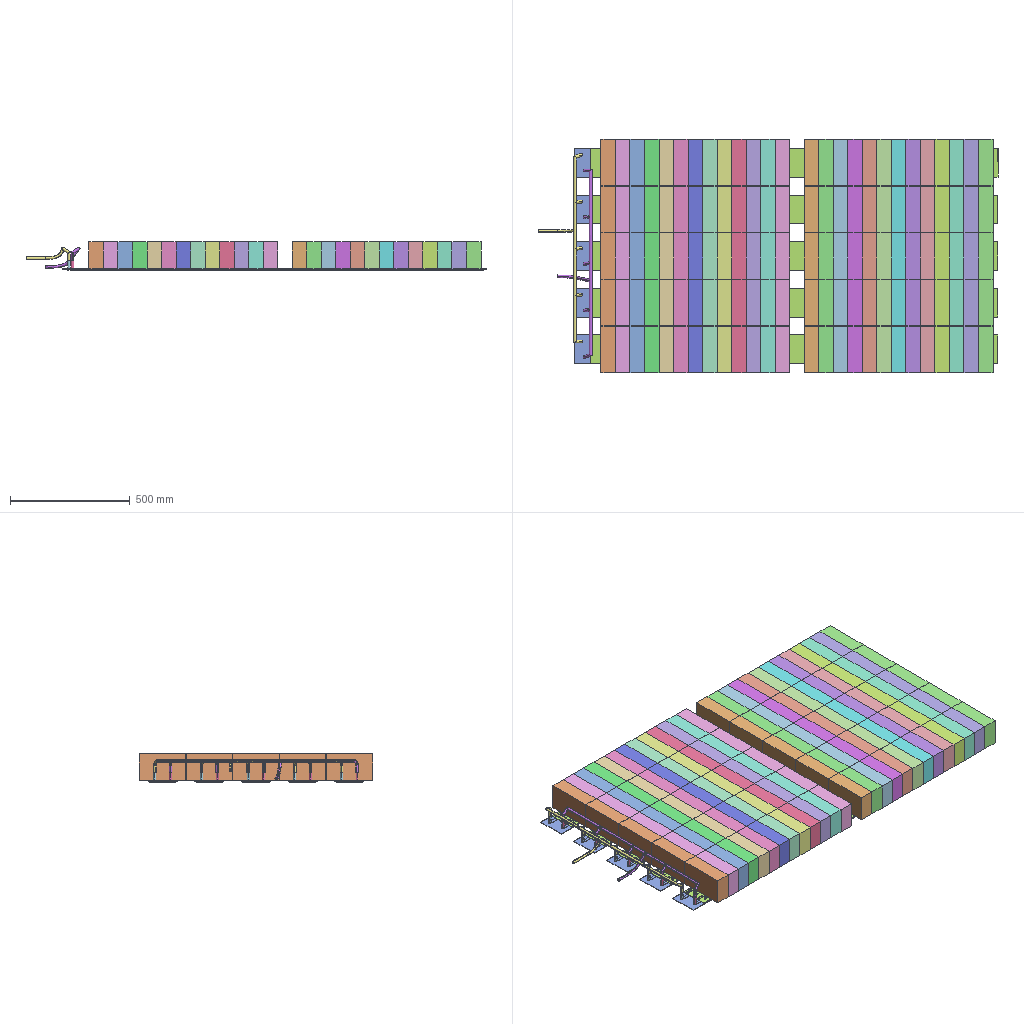Assembly | SolidWorks | 33 different items | 157 placed | box 1923 x 975 x 120 mm
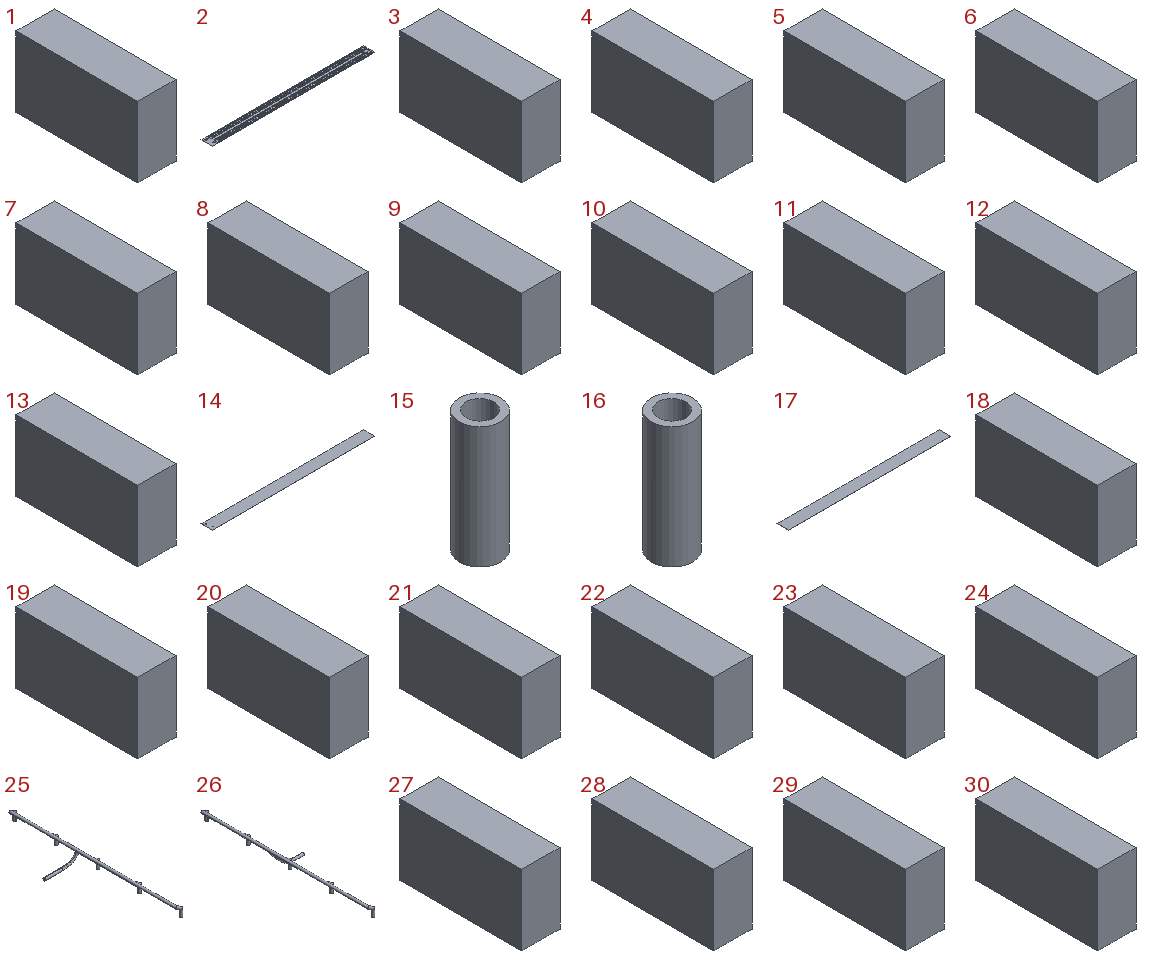Parts list (item | quantity | size | volume | features):
1 | x5 | 60.7 x 194.65 x 112.8 mm | 1332761 mm3 | features BaseBody 1
2 | x5 | 1768 x 120 x 5 mm | 283720 mm3 | features ICE 7, LPattern 2, BaseBody 1
3 | x5 | 60.7 x 194.65 x 112.8 mm | 1332761 mm3 | features BaseBody 1
4 | x5 | 60.7 x 194.65 x 112.8 mm | 1332761 mm3 | features BaseBody 1
5 | x5 | 60.7 x 194.65 x 112.8 mm | 1332761 mm3 | features BaseBody 1
6 | x5 | 60.7 x 194.65 x 112.8 mm | 1332761 mm3 | features BaseBody 1
7 | x5 | 60.7 x 194.65 x 112.8 mm | 1332761 mm3 | features BaseBody 1
8 | x5 | 60.7 x 194.65 x 112.8 mm | 1332761 mm3 | features BaseBody 1
9 | x5 | 60.7 x 194.65 x 112.8 mm | 1332761 mm3 | features BaseBody 1
10 | x5 | 60.7 x 194.65 x 112.8 mm | 1332761 mm3 | features BaseBody 1
11 | x5 | 60.7 x 194.65 x 112.8 mm | 1332761 mm3 | features BaseBody 1
12 | x5 | 60.7 x 194.65 x 112.8 mm | 1332761 mm3 | features BaseBody 1
13 | x5 | 60.7 x 194.65 x 112.8 mm | 1332761 mm3 | features BaseBody 1
14 | x5 | 1768 x 120 x 1 mm | 211934 mm3 | features BaseBody 1
15 | x5 | 12 x 12 x 35 mm | 2199 mm3 | features BaseBody 1
16 | x5 | 12 x 12 x 35 mm | 2199 mm3 | features BaseBody 1
17 | x5 | 1703 x 120 x 1 mm | 204360 mm3 | features BaseBody 1
18 | x5 | 60.7 x 194.65 x 112.8 mm | 1332761 mm3 | features BaseBody 1
19 | x5 | 60.7 x 194.65 x 112.8 mm | 1332761 mm3 | features BaseBody 1
20 | x5 | 60.7 x 194.65 x 112.8 mm | 1332761 mm3 | features BaseBody 1
21 | x5 | 60.7 x 194.65 x 112.8 mm | 1332761 mm3 | features BaseBody 1
22 | x5 | 60.7 x 194.65 x 112.8 mm | 1332761 mm3 | features BaseBody 1
23 | x5 | 60.7 x 194.65 x 112.8 mm | 1332761 mm3 | features BaseBody 1
24 | x5 | 60.7 x 194.65 x 112.8 mm | 1332761 mm3 | features BaseBody 1
25 | x1 | 185.606 x 792 x 56.756 mm | 78943 mm3 | features Sweep 5, 3DProfileFeature 2
26 | x1 | 146.397 x 792 x 87.372 mm | 78940 mm3 | features Sweep 5, 3DProfileFeature 2
27 | x5 | 60.7 x 194.65 x 112.8 mm | 1332761 mm3 | features BaseBody 1
28 | x5 | 60.7 x 194.65 x 112.8 mm | 1332761 mm3 | features BaseBody 1
29 | x5 | 60.7 x 194.65 x 112.8 mm | 1332761 mm3 | features BaseBody 1
30 | x5 | 60.7 x 194.65 x 112.8 mm | 1332761 mm3 | features BaseBody 1
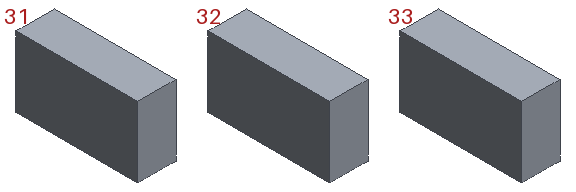31 | x5 | 60.7 x 194.65 x 112.8 mm | 1332761 mm3 | features BaseBody 1
32 | x5 | 60.7 x 194.65 x 112.8 mm | 1332761 mm3 | features BaseBody 1
33 | x5 | 60.7 x 194.65 x 112.8 mm | 1332761 mm3 | features BaseBody 1
Mates (type | each side: item.copy, entity, surface, feature):
Concentric | 16.1 face cylinder Imported1 | 25.1 face cylinder Sweep-Thin1
Concentric | 16.2 face cylinder Imported1 | 25.1 face cylinder Sweep-Thin1
Concentric | 15.1 face cylinder Imported1 | 26.1 face cylinder Sweep-Thin1
Concentric | 15.2 face cylinder Imported1 | 26.1 face cylinder Sweep-Thin4
Coincident | 15.1 face plane Imported1 | 26.1 face plane Sweep-Thin1
Coincident | 16.1 face plane Imported1 | 25.1 face plane Sweep-Thin1